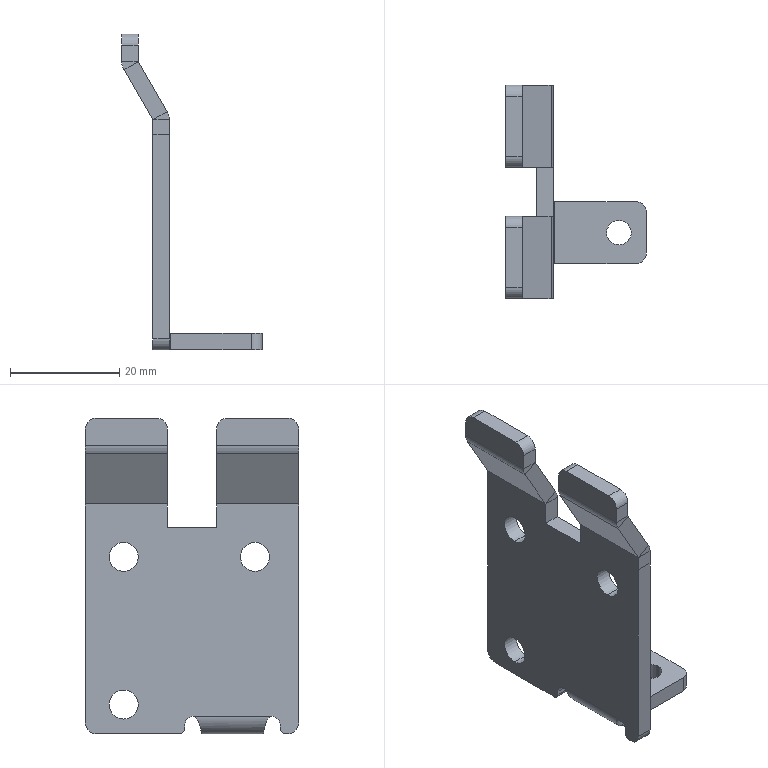Part | NX | features solid 2 | 1 solid | 78 faces | box 25.7 x 39 x 57.723 mm | volume 6585 mm3 | plane 46 | cylinder 30 | spline 2 | commonest cylinder face diameters 4 x8 5.3 x6 0.05 x2 0.095 x2 2 x2 3 x2